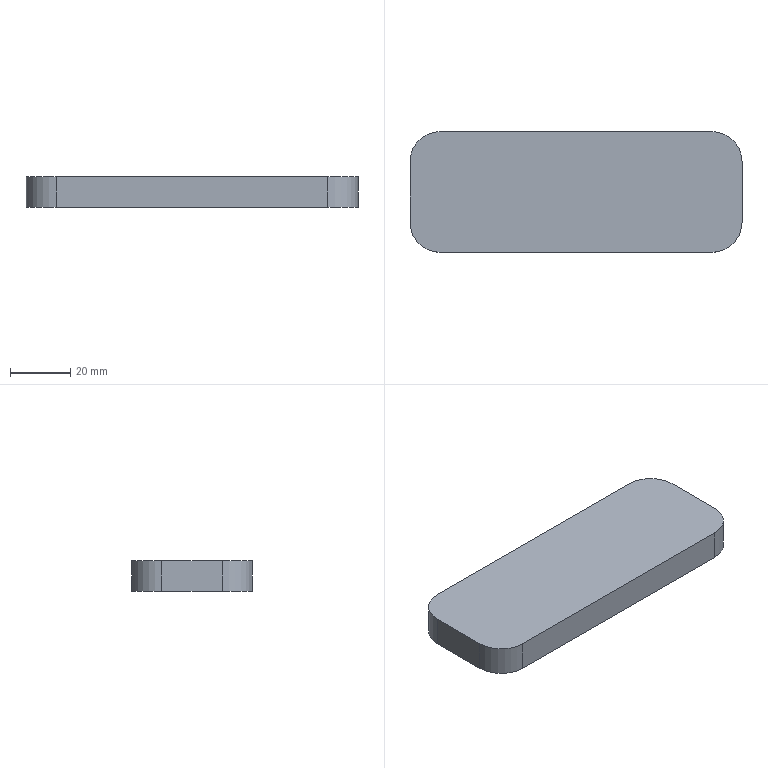Part | STEP file | SL2-MOLD_id18_xmt_txt | 1 solid | 10 faces | box 110 x 40 x 10 mm | volume 43142 mm3 | plane 6 | cylinder 4 | commonest cylinder face diameters 20 x4
STEP:
#1=CARTESIAN_POINT('',(-55.,-145.,20.));
#2=VERTEX_POINT('',#1);
#3=CARTESIAN_POINT('',(-55.,-125.,20.));
#4=VERTEX_POINT('',#3);
#5=CARTESIAN_POINT('',(-55.,-155.,20.));
#6=DIRECTION('',(0.,1.,0.));
#7=VECTOR('',#6,1.);
#8=LINE('',#5,#7);
#9=EDGE_CURVE('',#2,#4,#8,.T.);
#10=ORIENTED_EDGE('',*,*,#9,.F.);
#11=CARTESIAN_POINT('',(-55.,-145.,30.));
#12=VERTEX_POINT('',#11);
#13=CARTESIAN_POINT('',(-55.,-145.,20.));
#14=DIRECTION('',(0.,0.,1.));
#15=VECTOR('',#14,1.);
#16=LINE('',#13,#15);
#17=EDGE_CURVE('',#2,#12,#16,.T.);
#18=ORIENTED_EDGE('',*,*,#17,.T.);
#19=CARTESIAN_POINT('',(-55.,-125.,30.));
#20=VERTEX_POINT('',#19);
#21=CARTESIAN_POINT('',(-55.,-155.,30.));
#22=DIRECTION('',(0.,1.,0.));
#23=VECTOR('',#22,1.);
#24=LINE('',#21,#23);
#25=EDGE_CURVE('',#12,#20,#24,.T.);
#26=ORIENTED_EDGE('',*,*,#25,.T.);
#27=CARTESIAN_POINT('',(-55.,-125.,20.));
#28=DIRECTION('',(0.,0.,-1.));
#29=VECTOR('',#28,1.);
#30=LINE('',#27,#29);
#31=EDGE_CURVE('',#20,#4,#30,.T.);
#32=ORIENTED_EDGE('',*,*,#31,.T.);
#33=EDGE_LOOP('',(#10,#18,#26,#32));
#34=FACE_OUTER_BOUND('',#33,.T.);
#35=CARTESIAN_POINT('',(-55.,-155.,20.));
#36=DIRECTION('',(1.,0.,0.));
#37=DIRECTION('',(0.,1.,0.));
#38=AXIS2_PLACEMENT_3D('',#35,#36,#37);
#39=PLANE('',#38);
#40=ADVANCED_FACE('',(#34),#39,.F.);
#41=CARTESIAN_POINT('',(-45.,-115.,20.));
#42=VERTEX_POINT('',#41);
#43=CARTESIAN_POINT('',(45.,-115.,20.));
#44=VERTEX_POINT('',#43);
#45=CARTESIAN_POINT('',(-55.,-115.,20.));
#46=DIRECTION('',(1.,0.,0.));
#47=VECTOR('',#46,1.);
#48=LINE('',#45,#47);
#49=EDGE_CURVE('',#42,#44,#48,.T.);
#50=ORIENTED_EDGE('',*,*,#49,.F.);
#51=CARTESIAN_POINT('',(-45.,-115.,30.));
#52=VERTEX_POINT('',#51);
#53=CARTESIAN_POINT('',(-45.,-115.,20.));
#54=DIRECTION('',(0.,0.,1.));
#55=VECTOR('',#54,1.);
#56=LINE('',#53,#55);
#57=EDGE_CURVE('',#42,#52,#56,.T.);
#58=ORIENTED_EDGE('',*,*,#57,.T.);
#59=CARTESIAN_POINT('',(45.,-115.,30.));
#60=VERTEX_POINT('',#59);
#61=CARTESIAN_POINT('',(-55.,-115.,30.));
#62=DIRECTION('',(1.,0.,0.));
#63=VECTOR('',#62,1.);
#64=LINE('',#61,#63);
#65=EDGE_CURVE('',#52,#60,#64,.T.);
#66=ORIENTED_EDGE('',*,*,#65,.T.);
#67=CARTESIAN_POINT('',(45.,-115.,20.));
#68=DIRECTION('',(0.,0.,-1.));
#69=VECTOR('',#68,1.);
#70=LINE('',#67,#69);
#71=EDGE_CURVE('',#60,#44,#70,.T.);
#72=ORIENTED_EDGE('',*,*,#71,.T.);
#73=EDGE_LOOP('',(#50,#58,#66,#72));
#74=FACE_OUTER_BOUND('',#73,.T.);
#75=CARTESIAN_POINT('',(-55.,-115.,20.));
#76=DIRECTION('',(0.,-1.,0.));
#77=DIRECTION('',(0.,0.,-1.));
#78=AXIS2_PLACEMENT_3D('',#75,#76,#77);
#79=PLANE('',#78);
#80=ADVANCED_FACE('',(#74),#79,.F.);
#81=CARTESIAN_POINT('',(55.,-125.,20.));
#82=VERTEX_POINT('',#81);
#83=CARTESIAN_POINT('',(55.,-145.,20.));
#84=VERTEX_POINT('',#83);
#85=CARTESIAN_POINT('',(55.,-115.,20.));
#86=DIRECTION('',(0.,-1.,0.));
#87=VECTOR('',#86,1.);
#88=LINE('',#85,#87);
#89=EDGE_CURVE('',#82,#84,#88,.T.);
#90=ORIENTED_EDGE('',*,*,#89,.F.);
#91=CARTESIAN_POINT('',(55.,-125.,30.));
#92=VERTEX_POINT('',#91);
#93=CARTESIAN_POINT('',(55.,-125.,20.));
#94=DIRECTION('',(0.,0.,1.));
#95=VECTOR('',#94,1.);
#96=LINE('',#93,#95);
#97=EDGE_CURVE('',#82,#92,#96,.T.);
#98=ORIENTED_EDGE('',*,*,#97,.T.);
#99=CARTESIAN_POINT('',(55.,-145.,30.));
#100=VERTEX_POINT('',#99);
#101=CARTESIAN_POINT('',(55.,-115.,30.));
#102=DIRECTION('',(0.,-1.,0.));
#103=VECTOR('',#102,1.);
#104=LINE('',#101,#103);
#105=EDGE_CURVE('',#92,#100,#104,.T.);
#106=ORIENTED_EDGE('',*,*,#105,.T.);
#107=CARTESIAN_POINT('',(55.,-145.,20.));
#108=DIRECTION('',(0.,0.,-1.));
#109=VECTOR('',#108,1.);
#110=LINE('',#107,#109);
#111=EDGE_CURVE('',#100,#84,#110,.T.);
#112=ORIENTED_EDGE('',*,*,#111,.T.);
#113=EDGE_LOOP('',(#90,#98,#106,#112));
#114=FACE_OUTER_BOUND('',#113,.T.);
#115=CARTESIAN_POINT('',(55.,-115.,20.));
#116=DIRECTION('',(-1.,0.,0.));
#117=DIRECTION('',(0.,-1.,0.));
#118=AXIS2_PLACEMENT_3D('',#115,#116,#117);
#119=PLANE('',#118);
#120=ADVANCED_FACE('',(#114),#119,.F.);
#121=CARTESIAN_POINT('',(45.,-155.,30.));
#122=VERTEX_POINT('',#121);
#123=CARTESIAN_POINT('',(-45.,-155.,30.));
#124=VERTEX_POINT('',#123);
#125=CARTESIAN_POINT('',(55.,-155.,30.));
#126=DIRECTION('',(-1.,0.,0.));
#127=VECTOR('',#126,1.);
#128=LINE('',#125,#127);
#129=EDGE_CURVE('',#122,#124,#128,.T.);
#130=ORIENTED_EDGE('',*,*,#129,.T.);
#131=CARTESIAN_POINT('',(-45.,-155.,20.));
#132=VERTEX_POINT('',#131);
#133=CARTESIAN_POINT('',(-45.,-155.,20.));
#134=DIRECTION('',(0.,0.,-1.));
#135=VECTOR('',#134,1.);
#136=LINE('',#133,#135);
#137=EDGE_CURVE('',#124,#132,#136,.T.);
#138=ORIENTED_EDGE('',*,*,#137,.T.);
#139=CARTESIAN_POINT('',(45.,-155.,20.));
#140=VERTEX_POINT('',#139);
#141=CARTESIAN_POINT('',(55.,-155.,20.));
#142=DIRECTION('',(-1.,0.,0.));
#143=VECTOR('',#142,1.);
#144=LINE('',#141,#143);
#145=EDGE_CURVE('',#140,#132,#144,.T.);
#146=ORIENTED_EDGE('',*,*,#145,.F.);
#147=CARTESIAN_POINT('',(45.,-155.,20.));
#148=DIRECTION('',(0.,0.,1.));
#149=VECTOR('',#148,1.);
#150=LINE('',#147,#149);
#151=EDGE_CURVE('',#140,#122,#150,.T.);
#152=ORIENTED_EDGE('',*,*,#151,.T.);
#153=EDGE_LOOP('',(#130,#138,#146,#152));
#154=FACE_OUTER_BOUND('',#153,.T.);
#155=CARTESIAN_POINT('',(55.,-155.,20.));
#156=DIRECTION('',(0.,1.,0.));
#157=DIRECTION('',(0.,0.,1.));
#158=AXIS2_PLACEMENT_3D('',#155,#156,#157);
#159=PLANE('',#158);
#160=ADVANCED_FACE('',(#154),#159,.F.);
#161=ORIENTED_EDGE('',*,*,#145,.T.);
#162=CARTESIAN_POINT('',(-45.,-145.,20.));
#163=DIRECTION('',(0.,0.,-1.));
#164=DIRECTION('',(-1.,0.,0.));
#165=AXIS2_PLACEMENT_3D('',#162,#163,#164);
#166=CIRCLE('',#165,10.);
#167=EDGE_CURVE('',#132,#2,#166,.T.);
#168=ORIENTED_EDGE('',*,*,#167,.T.);
#169=ORIENTED_EDGE('',*,*,#9,.T.);
#170=CARTESIAN_POINT('',(-45.,-125.,20.));
#171=DIRECTION('',(0.,0.,-1.));
#172=DIRECTION('',(-1.,0.,0.));
#173=AXIS2_PLACEMENT_3D('',#170,#171,#172);
#174=CIRCLE('',#173,10.);
#175=EDGE_CURVE('',#4,#42,#174,.T.);
#176=ORIENTED_EDGE('',*,*,#175,.T.);
#177=ORIENTED_EDGE('',*,*,#49,.T.);
#178=CARTESIAN_POINT('',(45.,-125.,20.));
#179=DIRECTION('',(0.,0.,-1.));
#180=DIRECTION('',(-1.,0.,0.));
#181=AXIS2_PLACEMENT_3D('',#178,#179,#180);
#182=CIRCLE('',#181,10.);
#183=EDGE_CURVE('',#44,#82,#182,.T.);
#184=ORIENTED_EDGE('',*,*,#183,.T.);
#185=ORIENTED_EDGE('',*,*,#89,.T.);
#186=CARTESIAN_POINT('',(45.,-145.,20.));
#187=DIRECTION('',(0.,0.,-1.));
#188=DIRECTION('',(-1.,0.,0.));
#189=AXIS2_PLACEMENT_3D('',#186,#187,#188);
#190=CIRCLE('',#189,10.);
#191=EDGE_CURVE('',#84,#140,#190,.T.);
#192=ORIENTED_EDGE('',*,*,#191,.T.);
#193=EDGE_LOOP('',(#161,#168,#169,#176,#177,#184,#185,#192));
#194=FACE_OUTER_BOUND('',#193,.T.);
#195=CARTESIAN_POINT('',(0.,0.,20.));
#196=DIRECTION('',(0.,0.,-1.));
#197=DIRECTION('',(-1.,0.,0.));
#198=AXIS2_PLACEMENT_3D('',#195,#196,#197);
#199=PLANE('',#198);
#200=ADVANCED_FACE('',(#194),#199,.T.);
#201=ORIENTED_EDGE('',*,*,#25,.F.);
#202=CARTESIAN_POINT('',(-45.,-145.,30.));
#203=DIRECTION('',(0.,0.,1.));
#204=DIRECTION('',(-1.,0.,0.));
#205=AXIS2_PLACEMENT_3D('',#202,#203,#204);
#206=CIRCLE('',#205,10.);
#207=EDGE_CURVE('',#12,#124,#206,.T.);
#208=ORIENTED_EDGE('',*,*,#207,.T.);
#209=ORIENTED_EDGE('',*,*,#129,.F.);
#210=CARTESIAN_POINT('',(45.,-145.,30.));
#211=DIRECTION('',(0.,0.,1.));
#212=DIRECTION('',(-1.,0.,0.));
#213=AXIS2_PLACEMENT_3D('',#210,#211,#212);
#214=CIRCLE('',#213,10.);
#215=EDGE_CURVE('',#122,#100,#214,.T.);
#216=ORIENTED_EDGE('',*,*,#215,.T.);
#217=ORIENTED_EDGE('',*,*,#105,.F.);
#218=CARTESIAN_POINT('',(45.,-125.,30.));
#219=DIRECTION('',(0.,0.,1.));
#220=DIRECTION('',(-1.,0.,0.));
#221=AXIS2_PLACEMENT_3D('',#218,#219,#220);
#222=CIRCLE('',#221,10.);
#223=EDGE_CURVE('',#92,#60,#222,.T.);
#224=ORIENTED_EDGE('',*,*,#223,.T.);
#225=ORIENTED_EDGE('',*,*,#65,.F.);
#226=CARTESIAN_POINT('',(-45.,-125.,30.));
#227=DIRECTION('',(0.,0.,1.));
#228=DIRECTION('',(-1.,0.,0.));
#229=AXIS2_PLACEMENT_3D('',#226,#227,#228);
#230=CIRCLE('',#229,10.);
#231=EDGE_CURVE('',#52,#20,#230,.T.);
#232=ORIENTED_EDGE('',*,*,#231,.T.);
#233=EDGE_LOOP('',(#201,#208,#209,#216,#217,#224,#225,#232));
#234=FACE_OUTER_BOUND('',#233,.T.);
#235=CARTESIAN_POINT('',(0.,0.,30.));
#236=DIRECTION('',(0.,0.,-1.));
#237=DIRECTION('',(-1.,0.,0.));
#238=AXIS2_PLACEMENT_3D('',#235,#236,#237);
#239=PLANE('',#238);
#240=ADVANCED_FACE('',(#234),#239,.F.);
#241=ORIENTED_EDGE('',*,*,#167,.F.);
#242=ORIENTED_EDGE('',*,*,#137,.F.);
#243=ORIENTED_EDGE('',*,*,#207,.F.);
#244=ORIENTED_EDGE('',*,*,#17,.F.);
#245=EDGE_LOOP('',(#241,#242,#243,#244));
#246=FACE_OUTER_BOUND('',#245,.T.);
#247=CARTESIAN_POINT('',(-45.,-145.,20.));
#248=DIRECTION('',(0.,0.,1.));
#249=DIRECTION('',(1.,0.,0.));
#250=AXIS2_PLACEMENT_3D('',#247,#248,#249);
#251=CYLINDRICAL_SURFACE('',#250,10.);
#252=ADVANCED_FACE('',(#246),#251,.T.);
#253=ORIENTED_EDGE('',*,*,#175,.F.);
#254=ORIENTED_EDGE('',*,*,#31,.F.);
#255=ORIENTED_EDGE('',*,*,#231,.F.);
#256=ORIENTED_EDGE('',*,*,#57,.F.);
#257=EDGE_LOOP('',(#253,#254,#255,#256));
#258=FACE_OUTER_BOUND('',#257,.T.);
#259=CARTESIAN_POINT('',(-45.,-125.,20.));
#260=DIRECTION('',(0.,0.,1.));
#261=DIRECTION('',(1.,0.,0.));
#262=AXIS2_PLACEMENT_3D('',#259,#260,#261);
#263=CYLINDRICAL_SURFACE('',#262,10.);
#264=ADVANCED_FACE('',(#258),#263,.T.);
#265=ORIENTED_EDGE('',*,*,#183,.F.);
#266=ORIENTED_EDGE('',*,*,#71,.F.);
#267=ORIENTED_EDGE('',*,*,#223,.F.);
#268=ORIENTED_EDGE('',*,*,#97,.F.);
#269=EDGE_LOOP('',(#265,#266,#267,#268));
#270=FACE_OUTER_BOUND('',#269,.T.);
#271=CARTESIAN_POINT('',(45.,-125.,20.));
#272=DIRECTION('',(0.,0.,1.));
#273=DIRECTION('',(1.,0.,0.));
#274=AXIS2_PLACEMENT_3D('',#271,#272,#273);
#275=CYLINDRICAL_SURFACE('',#274,10.);
#276=ADVANCED_FACE('',(#270),#275,.T.);
#277=ORIENTED_EDGE('',*,*,#191,.F.);
#278=ORIENTED_EDGE('',*,*,#111,.F.);
#279=ORIENTED_EDGE('',*,*,#215,.F.);
#280=ORIENTED_EDGE('',*,*,#151,.F.);
#281=EDGE_LOOP('',(#277,#278,#279,#280));
#282=FACE_OUTER_BOUND('',#281,.T.);
#283=CARTESIAN_POINT('',(45.,-145.,20.));
#284=DIRECTION('',(0.,0.,1.));
#285=DIRECTION('',(1.,0.,0.));
#286=AXIS2_PLACEMENT_3D('',#283,#284,#285);
#287=CYLINDRICAL_SURFACE('',#286,10.);
#288=ADVANCED_FACE('',(#282),#287,.T.);
#289=CLOSED_SHELL('',(#40,#80,#120,#160,#200,#240,#252,#264,#276,#288));
#290=MANIFOLD_SOLID_BREP('',#289);
#291=(LENGTH_UNIT()NAMED_UNIT(*)SI_UNIT(.MILLI.,.METRE.));
#292=UNCERTAINTY_MEASURE_WITH_UNIT(LENGTH_MEASURE(0.00002),#291,'','');
#293=(NAMED_UNIT(*)PLANE_ANGLE_UNIT()SI_UNIT($,.RADIAN.));
#294=PLANE_ANGLE_MEASURE_WITH_UNIT(PLANE_ANGLE_MEASURE(0.01745),#293);
#295=DIMENSIONAL_EXPONENTS(0.,0.,0.,0.,0.,0.,0.);
#296=(CONVERSION_BASED_UNIT('DEGREE',#294)NAMED_UNIT(#295)PLANE_ANGLE_UNIT());
#297=(NAMED_UNIT(*)SI_UNIT($,.STERADIAN.)SOLID_ANGLE_UNIT());
#298=(GEOMETRIC_REPRESENTATION_CONTEXT(3)GLOBAL_UNCERTAINTY_ASSIGNED_CONTEXT((#292))GLOBAL_UNIT_ASSIGNED_CONTEXT((#291,#296,#297))REPRESENTATION_CONTEXT('',''));
#299=ADVANCED_BREP_SHAPE_REPRESENTATION('',(#290),#298);